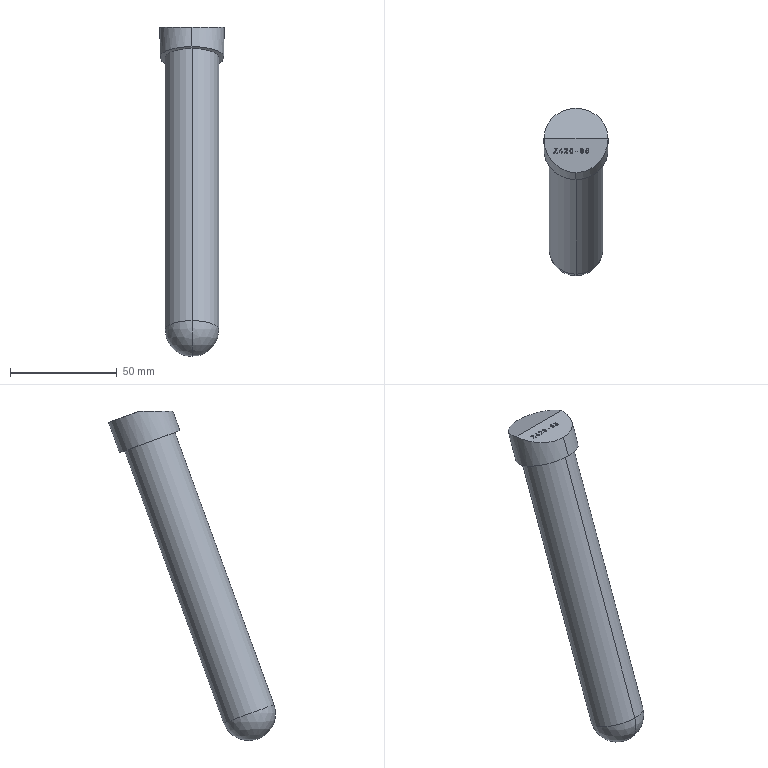Part | Creo | 1 solid | 133 faces | box 30 x 78.048 x 153.865 mm | volume 80356 mm3 | other 81 | plane 44 | cylinder 6 | sphere 2 | commonest cylinder face diameters 25 x2 30 x2 1.927 x1 30.388 x1